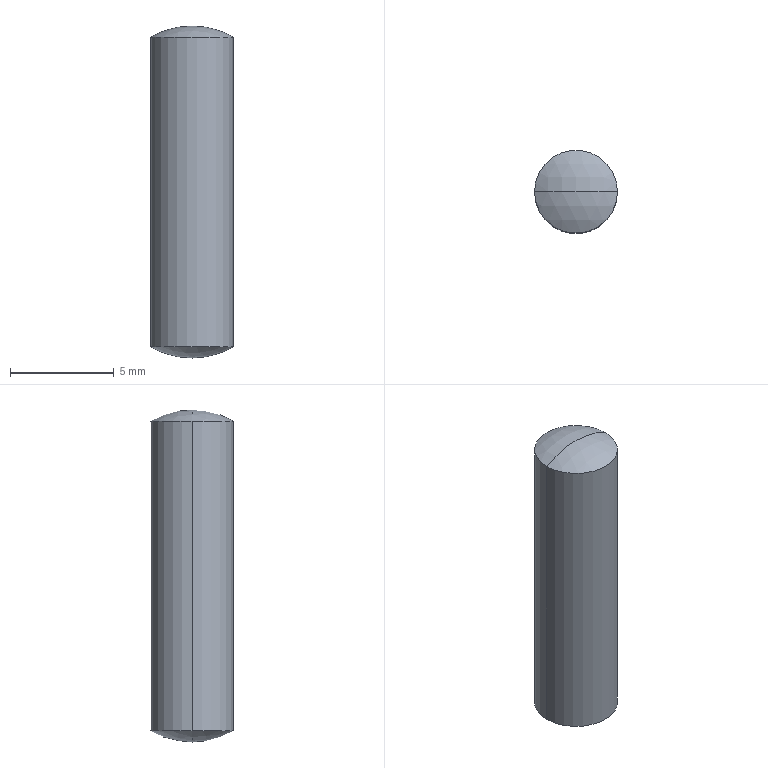Part | SolidWorks | features Attribute 1, Revolution 1 | 1 solid | 6 faces | box 4 x 4 x 16 mm | volume 194.489 mm3 | sphere 4 | cylinder 2 | commonest cylinder face diameters 4 x2
STEP:
#1=CARTESIAN_POINT('',(-2.,0.,7.464));
#2=VERTEX_POINT('',#1);
#3=CARTESIAN_POINT('',(2.,0.,7.464));
#4=VERTEX_POINT('',#3);
#5=CARTESIAN_POINT('',(0.,0.,7.464));
#6=DIRECTION('',(0.,0.,-1.));
#7=DIRECTION('',(-1.,0.,0.));
#8=AXIS2_PLACEMENT_3D('',#5,#6,#7);
#9=CIRCLE('',#8,2.);
#10=EDGE_CURVE('',#2,#4,#9,.T.);
#11=ORIENTED_EDGE('',*,*,#10,.T.);
#12=CARTESIAN_POINT('',(2.,0.,-7.464));
#13=VERTEX_POINT('',#12);
#14=CARTESIAN_POINT('',(2.,0.,-47.537));
#15=DIRECTION('',(0.,0.,-1.));
#16=VECTOR('',#15,1000.);
#17=LINE('',#14,#16);
#18=EDGE_CURVE('',#4,#13,#17,.T.);
#19=ORIENTED_EDGE('',*,*,#18,.T.);
#20=CARTESIAN_POINT('',(-2.,0.,-7.464));
#21=VERTEX_POINT('',#20);
#22=CARTESIAN_POINT('',(0.,0.,-7.464));
#23=DIRECTION('',(0.,0.,-1.));
#24=DIRECTION('',(-1.,0.,0.));
#25=AXIS2_PLACEMENT_3D('',#22,#23,#24);
#26=CIRCLE('',#25,2.);
#27=EDGE_CURVE('',#21,#13,#26,.T.);
#28=ORIENTED_EDGE('',*,*,#27,.F.);
#29=CARTESIAN_POINT('',(-2.,0.,-47.537));
#30=DIRECTION('',(0.,0.,-1.));
#31=VECTOR('',#30,1000.);
#32=LINE('',#29,#31);
#33=EDGE_CURVE('',#2,#21,#32,.T.);
#34=ORIENTED_EDGE('',*,*,#33,.F.);
#35=EDGE_LOOP('',(#11,#19,#28,#34));
#36=FACE_OUTER_BOUND('',#35,.T.);
#37=CARTESIAN_POINT('',(0.,0.,-47.537));
#38=DIRECTION('',(0.,0.,-1.));
#39=DIRECTION('',(-1.,0.,0.));
#40=AXIS2_PLACEMENT_3D('',#37,#38,#39);
#41=CYLINDRICAL_SURFACE('',#40,2.);
#42=ADVANCED_FACE('',(#36),#41,.T.);
#43=CARTESIAN_POINT('',(0.,0.,8.));
#44=VERTEX_POINT('',#43);
#45=CARTESIAN_POINT('',(0.,0.,4.));
#46=DIRECTION('',(0.,1.,0.));
#47=DIRECTION('',(0.,0.,1.));
#48=AXIS2_PLACEMENT_3D('',#45,#46,#47);
#49=CIRCLE('',#48,4.);
#50=EDGE_CURVE('',#44,#4,#49,.T.);
#51=ORIENTED_EDGE('',*,*,#50,.F.);
#52=CARTESIAN_POINT('',(0.,0.,4.));
#53=DIRECTION('',(0.,-1.,0.));
#54=DIRECTION('',(1.,0.,0.));
#55=AXIS2_PLACEMENT_3D('',#52,#53,#54);
#56=CIRCLE('',#55,4.);
#57=EDGE_CURVE('',#44,#2,#56,.T.);
#58=ORIENTED_EDGE('',*,*,#57,.T.);
#59=CARTESIAN_POINT('',(0.,0.,7.464));
#60=DIRECTION('',(0.,0.,-1.));
#61=DIRECTION('',(-1.,0.,0.));
#62=AXIS2_PLACEMENT_3D('',#59,#60,#61);
#63=CIRCLE('',#62,2.);
#64=EDGE_CURVE('',#4,#2,#63,.T.);
#65=ORIENTED_EDGE('',*,*,#64,.F.);
#66=EDGE_LOOP('',(#51,#58,#65));
#67=FACE_OUTER_BOUND('',#66,.T.);
#68=CARTESIAN_POINT('',(0.,0.,4.));
#69=DIRECTION('',(0.,-1.,0.));
#70=DIRECTION('',(1.,0.,0.));
#71=AXIS2_PLACEMENT_3D('',#68,#69,#70);
#72=SPHERICAL_SURFACE('',#71,4.);
#73=ADVANCED_FACE('',(#67),#72,.T.);
#74=ORIENTED_EDGE('',*,*,#27,.T.);
#75=CARTESIAN_POINT('',(0.,0.,-8.));
#76=VERTEX_POINT('',#75);
#77=CARTESIAN_POINT('',(0.,0.,-4.));
#78=DIRECTION('',(0.,1.,0.));
#79=DIRECTION('',(-1.,0.,0.));
#80=AXIS2_PLACEMENT_3D('',#77,#78,#79);
#81=CIRCLE('',#80,4.);
#82=EDGE_CURVE('',#13,#76,#81,.T.);
#83=ORIENTED_EDGE('',*,*,#82,.T.);
#84=CARTESIAN_POINT('',(0.,0.,-4.));
#85=DIRECTION('',(0.,-1.,0.));
#86=DIRECTION('',(0.,0.,-1.));
#87=AXIS2_PLACEMENT_3D('',#84,#85,#86);
#88=CIRCLE('',#87,4.);
#89=EDGE_CURVE('',#21,#76,#88,.T.);
#90=ORIENTED_EDGE('',*,*,#89,.F.);
#91=EDGE_LOOP('',(#74,#83,#90));
#92=FACE_OUTER_BOUND('',#91,.T.);
#93=CARTESIAN_POINT('',(0.,0.,-4.));
#94=DIRECTION('',(0.,1.,0.));
#95=DIRECTION('',(-1.,0.,0.));
#96=AXIS2_PLACEMENT_3D('',#93,#94,#95);
#97=SPHERICAL_SURFACE('',#96,4.);
#98=ADVANCED_FACE('',(#92),#97,.T.);
#99=ORIENTED_EDGE('',*,*,#82,.F.);
#100=CARTESIAN_POINT('',(0.,0.,-7.464));
#101=DIRECTION('',(0.,0.,-1.));
#102=DIRECTION('',(-1.,0.,0.));
#103=AXIS2_PLACEMENT_3D('',#100,#101,#102);
#104=CIRCLE('',#103,2.);
#105=EDGE_CURVE('',#13,#21,#104,.T.);
#106=ORIENTED_EDGE('',*,*,#105,.T.);
#107=ORIENTED_EDGE('',*,*,#89,.T.);
#108=EDGE_LOOP('',(#99,#106,#107));
#109=FACE_OUTER_BOUND('',#108,.T.);
#110=CARTESIAN_POINT('',(0.,0.,-4.));
#111=DIRECTION('',(0.,1.,0.));
#112=DIRECTION('',(-1.,0.,0.));
#113=AXIS2_PLACEMENT_3D('',#110,#111,#112);
#114=SPHERICAL_SURFACE('',#113,4.);
#115=ADVANCED_FACE('',(#109),#114,.T.);
#116=ORIENTED_EDGE('',*,*,#57,.F.);
#117=ORIENTED_EDGE('',*,*,#50,.T.);
#118=ORIENTED_EDGE('',*,*,#10,.F.);
#119=EDGE_LOOP('',(#116,#117,#118));
#120=FACE_OUTER_BOUND('',#119,.T.);
#121=CARTESIAN_POINT('',(0.,0.,4.));
#122=DIRECTION('',(0.,-1.,0.));
#123=DIRECTION('',(1.,0.,0.));
#124=AXIS2_PLACEMENT_3D('',#121,#122,#123);
#125=SPHERICAL_SURFACE('',#124,4.);
#126=ADVANCED_FACE('',(#120),#125,.T.);
#127=ORIENTED_EDGE('',*,*,#18,.F.);
#128=ORIENTED_EDGE('',*,*,#64,.T.);
#129=ORIENTED_EDGE('',*,*,#33,.T.);
#130=ORIENTED_EDGE('',*,*,#105,.F.);
#131=EDGE_LOOP('',(#127,#128,#129,#130));
#132=FACE_OUTER_BOUND('',#131,.T.);
#133=CARTESIAN_POINT('',(0.,0.,-47.537));
#134=DIRECTION('',(0.,0.,-1.));
#135=DIRECTION('',(-1.,0.,0.));
#136=AXIS2_PLACEMENT_3D('',#133,#134,#135);
#137=CYLINDRICAL_SURFACE('',#136,2.);
#138=ADVANCED_FACE('',(#132),#137,.T.);
#139=CLOSED_SHELL('',(#42,#73,#98,#115,#126,#138));
#140=MANIFOLD_SOLID_BREP('',#139);
#141=CARTESIAN_POINT('',(0.,0.,0.));
#142=DIRECTION('',(0.,0.,1.));
#143=DIRECTION('',(1.,0.,0.));
#144=AXIS2_PLACEMENT_3D('',#141,#142,#143);
#145=(LENGTH_UNIT()NAMED_UNIT(*)SI_UNIT(.MILLI.,.METRE.));
#146=UNCERTAINTY_MEASURE_WITH_UNIT(LENGTH_MEASURE(0.00001),#145,'','');
#147=(NAMED_UNIT(*)PLANE_ANGLE_UNIT()SI_UNIT($,.RADIAN.));
#148=(NAMED_UNIT(*)SI_UNIT($,.STERADIAN.)SOLID_ANGLE_UNIT());
#149=(GEOMETRIC_REPRESENTATION_CONTEXT(3)GLOBAL_UNCERTAINTY_ASSIGNED_CONTEXT((#146))GLOBAL_UNIT_ASSIGNED_CONTEXT((#145,#147,#148))REPRESENTATION_CONTEXT('',''));
#150=ADVANCED_BREP_SHAPE_REPRESENTATION('',(#140,#144),#149);